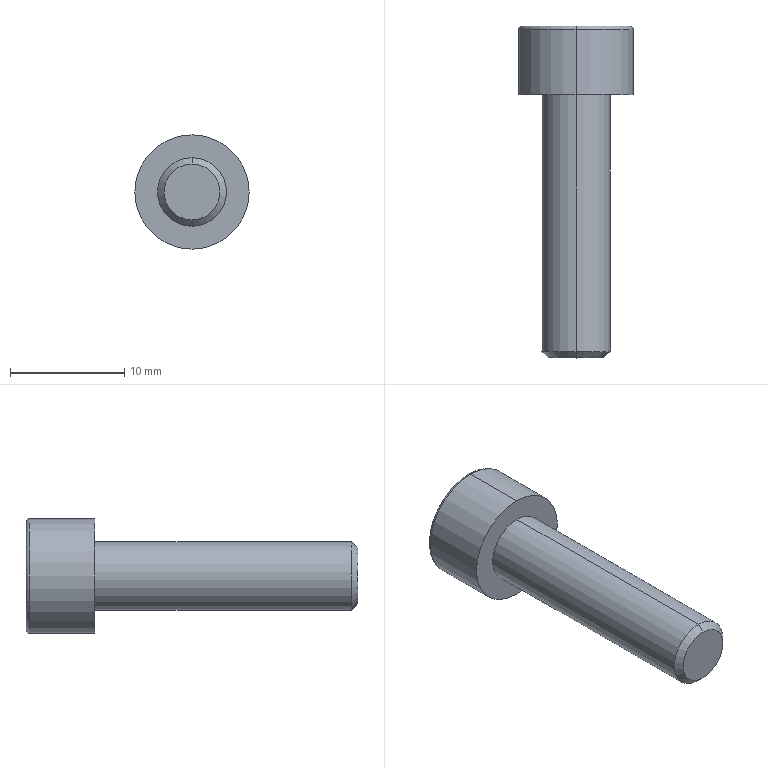Part | SolidWorks | features BaseBody 1 | 1 solid | 18 faces | box 10 x 29 x 10 mm | volume 1051 mm3 | plane 10 | cylinder 4 | cone 2 | torus 2 | commonest cylinder face diameters 6 x2 10 x2
STEP:
#1=CARTESIAN_POINT('',(0.,-23.,-2.445));
#2=VERTEX_POINT('',#1);
#3=CARTESIAN_POINT('',(0.,-23.,2.445));
#4=VERTEX_POINT('',#3);
#5=CARTESIAN_POINT('',(0.,-23.,0.));
#6=DIRECTION('',(0.,-1.,0.));
#7=DIRECTION('',(0.,0.,-1.));
#8=AXIS2_PLACEMENT_3D('',#5,#6,#7);
#9=CIRCLE('',#8,2.445);
#10=EDGE_CURVE('',#2,#4,#9,.T.);
#11=ORIENTED_EDGE('',*,*,#10,.F.);
#12=CARTESIAN_POINT('',(0.,-22.445,-3.));
#13=VERTEX_POINT('',#12);
#14=CARTESIAN_POINT('',(0.,-23.,-2.445));
#15=DIRECTION('',(0.,0.7071,-0.7071));
#16=VECTOR('',#15,1000.);
#17=LINE('',#14,#16);
#18=EDGE_CURVE('',#2,#13,#17,.T.);
#19=ORIENTED_EDGE('',*,*,#18,.T.);
#20=CARTESIAN_POINT('',(0.,-22.445,3.));
#21=VERTEX_POINT('',#20);
#22=CARTESIAN_POINT('',(0.,-22.445,0.));
#23=DIRECTION('',(0.,1.,0.));
#24=DIRECTION('',(0.,0.,-1.));
#25=AXIS2_PLACEMENT_3D('',#22,#23,#24);
#26=CIRCLE('',#25,3.);
#27=EDGE_CURVE('',#21,#13,#26,.T.);
#28=ORIENTED_EDGE('',*,*,#27,.F.);
#29=CARTESIAN_POINT('',(0.,-23.,2.445));
#30=DIRECTION('',(0.,0.7071,0.7071));
#31=VECTOR('',#30,1000.);
#32=LINE('',#29,#31);
#33=EDGE_CURVE('',#4,#21,#32,.T.);
#34=ORIENTED_EDGE('',*,*,#33,.F.);
#35=EDGE_LOOP('',(#11,#19,#28,#34));
#36=FACE_OUTER_BOUND('',#35,.T.);
#37=CARTESIAN_POINT('',(0.,-23.,0.));
#38=DIRECTION('',(0.,1.,0.));
#39=DIRECTION('',(0.,0.,1.));
#40=AXIS2_PLACEMENT_3D('',#37,#38,#39);
#41=CONICAL_SURFACE('',#40,2.445,0.7854);
#42=ADVANCED_FACE('',(#36),#41,.T.);
#43=ORIENTED_EDGE('',*,*,#27,.T.);
#44=CARTESIAN_POINT('',(0.,0.,-3.));
#45=VERTEX_POINT('',#44);
#46=CARTESIAN_POINT('',(0.,-23.,-3.));
#47=DIRECTION('',(0.,1.,0.));
#48=VECTOR('',#47,1000.);
#49=LINE('',#46,#48);
#50=EDGE_CURVE('',#13,#45,#49,.T.);
#51=ORIENTED_EDGE('',*,*,#50,.T.);
#52=CARTESIAN_POINT('',(0.,0.,3.));
#53=VERTEX_POINT('',#52);
#54=CARTESIAN_POINT('',(0.,0.,0.));
#55=DIRECTION('',(0.,-1.,0.));
#56=DIRECTION('',(0.,0.,1.));
#57=AXIS2_PLACEMENT_3D('',#54,#55,#56);
#58=CIRCLE('',#57,3.);
#59=EDGE_CURVE('',#45,#53,#58,.T.);
#60=ORIENTED_EDGE('',*,*,#59,.T.);
#61=CARTESIAN_POINT('',(0.,-23.,3.));
#62=DIRECTION('',(0.,1.,0.));
#63=VECTOR('',#62,1000.);
#64=LINE('',#61,#63);
#65=EDGE_CURVE('',#21,#53,#64,.T.);
#66=ORIENTED_EDGE('',*,*,#65,.F.);
#67=EDGE_LOOP('',(#43,#51,#60,#66));
#68=FACE_OUTER_BOUND('',#67,.T.);
#69=CARTESIAN_POINT('',(0.,-23.,0.));
#70=DIRECTION('',(0.,1.,0.));
#71=DIRECTION('',(0.,0.,1.));
#72=AXIS2_PLACEMENT_3D('',#69,#70,#71);
#73=CYLINDRICAL_SURFACE('',#72,3.);
#74=ADVANCED_FACE('',(#68),#73,.T.);
#75=CARTESIAN_POINT('',(0.,5.7,-5.));
#76=VERTEX_POINT('',#75);
#77=CARTESIAN_POINT('',(0.,5.7,5.));
#78=VERTEX_POINT('',#77);
#79=CARTESIAN_POINT('',(0.,5.7,0.));
#80=DIRECTION('',(0.,-1.,0.));
#81=DIRECTION('',(0.,0.,1.));
#82=AXIS2_PLACEMENT_3D('',#79,#80,#81);
#83=CIRCLE('',#82,5.);
#84=EDGE_CURVE('',#76,#78,#83,.T.);
#85=ORIENTED_EDGE('',*,*,#84,.F.);
#86=CARTESIAN_POINT('',(0.,6.,-4.7));
#87=VERTEX_POINT('',#86);
#88=CARTESIAN_POINT('',(0.,5.7,-4.7));
#89=DIRECTION('',(1.,0.,0.));
#90=DIRECTION('',(0.,0.,-1.));
#91=AXIS2_PLACEMENT_3D('',#88,#89,#90);
#92=CIRCLE('',#91,0.3);
#93=EDGE_CURVE('',#76,#87,#92,.T.);
#94=ORIENTED_EDGE('',*,*,#93,.T.);
#95=CARTESIAN_POINT('',(0.,6.,4.7));
#96=VERTEX_POINT('',#95);
#97=CARTESIAN_POINT('',(0.,6.,0.));
#98=DIRECTION('',(0.,1.,0.));
#99=DIRECTION('',(0.,0.,1.));
#100=AXIS2_PLACEMENT_3D('',#97,#98,#99);
#101=CIRCLE('',#100,4.7);
#102=EDGE_CURVE('',#96,#87,#101,.T.);
#103=ORIENTED_EDGE('',*,*,#102,.F.);
#104=CARTESIAN_POINT('',(0.,5.7,4.7));
#105=DIRECTION('',(-1.,0.,0.));
#106=DIRECTION('',(0.,0.,1.));
#107=AXIS2_PLACEMENT_3D('',#104,#105,#106);
#108=CIRCLE('',#107,0.3);
#109=EDGE_CURVE('',#78,#96,#108,.T.);
#110=ORIENTED_EDGE('',*,*,#109,.F.);
#111=EDGE_LOOP('',(#85,#94,#103,#110));
#112=FACE_OUTER_BOUND('',#111,.T.);
#113=CARTESIAN_POINT('',(0.,5.7,0.));
#114=DIRECTION('',(0.,1.,0.));
#115=DIRECTION('',(0.,0.,1.));
#116=AXIS2_PLACEMENT_3D('',#113,#114,#115);
#117=TOROIDAL_SURFACE('',#116,4.7,0.3);
#118=ADVANCED_FACE('',(#112),#117,.T.);
#119=ORIENTED_EDGE('',*,*,#84,.T.);
#120=CARTESIAN_POINT('',(0.,0.,5.));
#121=VERTEX_POINT('',#120);
#122=CARTESIAN_POINT('',(0.,6.,5.));
#123=DIRECTION('',(0.,-1.,0.));
#124=VECTOR('',#123,1000.);
#125=LINE('',#122,#124);
#126=EDGE_CURVE('',#78,#121,#125,.T.);
#127=ORIENTED_EDGE('',*,*,#126,.T.);
#128=CARTESIAN_POINT('',(0.,0.,-5.));
#129=VERTEX_POINT('',#128);
#130=CARTESIAN_POINT('',(0.,0.,0.));
#131=DIRECTION('',(0.,1.,0.));
#132=DIRECTION('',(0.,0.,1.));
#133=AXIS2_PLACEMENT_3D('',#130,#131,#132);
#134=CIRCLE('',#133,5.);
#135=EDGE_CURVE('',#121,#129,#134,.T.);
#136=ORIENTED_EDGE('',*,*,#135,.T.);
#137=CARTESIAN_POINT('',(0.,6.,-5.));
#138=DIRECTION('',(0.,-1.,0.));
#139=VECTOR('',#138,1000.);
#140=LINE('',#137,#139);
#141=EDGE_CURVE('',#76,#129,#140,.T.);
#142=ORIENTED_EDGE('',*,*,#141,.F.);
#143=EDGE_LOOP('',(#119,#127,#136,#142));
#144=FACE_OUTER_BOUND('',#143,.T.);
#145=CARTESIAN_POINT('',(0.,6.,0.));
#146=DIRECTION('',(0.,-1.,0.));
#147=DIRECTION('',(0.,0.,-1.));
#148=AXIS2_PLACEMENT_3D('',#145,#146,#147);
#149=CYLINDRICAL_SURFACE('',#148,5.);
#150=ADVANCED_FACE('',(#144),#149,.T.);
#151=CARTESIAN_POINT('',(0.,-23.,0.));
#152=DIRECTION('',(0.,-1.,0.));
#153=DIRECTION('',(0.,0.,-1.));
#154=AXIS2_PLACEMENT_3D('',#151,#152,#153);
#155=CIRCLE('',#154,2.445);
#156=EDGE_CURVE('',#4,#2,#155,.T.);
#157=ORIENTED_EDGE('',*,*,#156,.T.);
#158=ORIENTED_EDGE('',*,*,#10,.T.);
#159=EDGE_LOOP('',(#157,#158));
#160=FACE_OUTER_BOUND('',#159,.T.);
#161=CARTESIAN_POINT('',(0.,-23.,0.));
#162=DIRECTION('',(0.,-1.,0.));
#163=DIRECTION('',(0.,0.,-1.));
#164=AXIS2_PLACEMENT_3D('',#161,#162,#163);
#165=PLANE('',#164);
#166=ADVANCED_FACE('',(#160),#165,.T.);
#167=CARTESIAN_POINT('',(1.466,3.,2.54));
#168=VERTEX_POINT('',#167);
#169=CARTESIAN_POINT('',(2.933,3.,0.));
#170=VERTEX_POINT('',#169);
#171=CARTESIAN_POINT('',(1.466,3.,2.54));
#172=DIRECTION('',(0.5,0.,-0.866));
#173=VECTOR('',#172,1000.);
#174=LINE('',#171,#173);
#175=EDGE_CURVE('',#168,#170,#174,.T.);
#176=ORIENTED_EDGE('',*,*,#175,.T.);
#177=CARTESIAN_POINT('',(1.466,3.,-2.54));
#178=VERTEX_POINT('',#177);
#179=CARTESIAN_POINT('',(2.933,3.,0.));
#180=DIRECTION('',(-0.5,0.,-0.866));
#181=VECTOR('',#180,1000.);
#182=LINE('',#179,#181);
#183=EDGE_CURVE('',#170,#178,#182,.T.);
#184=ORIENTED_EDGE('',*,*,#183,.T.);
#185=CARTESIAN_POINT('',(-1.466,3.,-2.54));
#186=VERTEX_POINT('',#185);
#187=CARTESIAN_POINT('',(1.466,3.,-2.54));
#188=DIRECTION('',(-1.,0.,0.));
#189=VECTOR('',#188,1000.);
#190=LINE('',#187,#189);
#191=EDGE_CURVE('',#178,#186,#190,.T.);
#192=ORIENTED_EDGE('',*,*,#191,.T.);
#193=CARTESIAN_POINT('',(-2.933,3.,0.));
#194=VERTEX_POINT('',#193);
#195=CARTESIAN_POINT('',(-1.466,3.,-2.54));
#196=DIRECTION('',(-0.5,0.,0.866));
#197=VECTOR('',#196,1000.);
#198=LINE('',#195,#197);
#199=EDGE_CURVE('',#186,#194,#198,.T.);
#200=ORIENTED_EDGE('',*,*,#199,.T.);
#201=CARTESIAN_POINT('',(-1.466,3.,2.54));
#202=VERTEX_POINT('',#201);
#203=CARTESIAN_POINT('',(-2.933,3.,0.));
#204=DIRECTION('',(0.5,0.,0.866));
#205=VECTOR('',#204,1000.);
#206=LINE('',#203,#205);
#207=EDGE_CURVE('',#194,#202,#206,.T.);
#208=ORIENTED_EDGE('',*,*,#207,.T.);
#209=CARTESIAN_POINT('',(-1.466,3.,2.54));
#210=DIRECTION('',(1.,0.,0.));
#211=VECTOR('',#210,1000.);
#212=LINE('',#209,#211);
#213=EDGE_CURVE('',#202,#168,#212,.T.);
#214=ORIENTED_EDGE('',*,*,#213,.T.);
#215=EDGE_LOOP('',(#176,#184,#192,#200,#208,#214));
#216=FACE_OUTER_BOUND('',#215,.T.);
#217=CARTESIAN_POINT('',(0.,3.,0.));
#218=DIRECTION('',(0.,1.,0.));
#219=DIRECTION('',(1.,0.,0.));
#220=AXIS2_PLACEMENT_3D('',#217,#218,#219);
#221=PLANE('',#220);
#222=ADVANCED_FACE('',(#216),#221,.T.);
#223=CARTESIAN_POINT('',(2.933,6.,0.));
#224=VERTEX_POINT('',#223);
#225=CARTESIAN_POINT('',(1.466,6.,-2.54));
#226=VERTEX_POINT('',#225);
#227=CARTESIAN_POINT('',(2.933,6.,0.));
#228=DIRECTION('',(-0.5,0.,-0.866));
#229=VECTOR('',#228,1000.);
#230=LINE('',#227,#229);
#231=EDGE_CURVE('',#224,#226,#230,.T.);
#232=ORIENTED_EDGE('',*,*,#231,.T.);
#233=CARTESIAN_POINT('',(1.466,3.,-2.54));
#234=DIRECTION('',(0.,1.,0.));
#235=VECTOR('',#234,1000.);
#236=LINE('',#233,#235);
#237=EDGE_CURVE('',#178,#226,#236,.T.);
#238=ORIENTED_EDGE('',*,*,#237,.F.);
#239=ORIENTED_EDGE('',*,*,#183,.F.);
#240=CARTESIAN_POINT('',(2.933,3.,0.));
#241=DIRECTION('',(0.,1.,0.));
#242=VECTOR('',#241,1000.);
#243=LINE('',#240,#242);
#244=EDGE_CURVE('',#170,#224,#243,.T.);
#245=ORIENTED_EDGE('',*,*,#244,.T.);
#246=EDGE_LOOP('',(#232,#238,#239,#245));
#247=FACE_OUTER_BOUND('',#246,.T.);
#248=CARTESIAN_POINT('',(2.933,3.,0.));
#249=DIRECTION('',(0.866,0.,-0.5));
#250=DIRECTION('',(0.,-1.,0.));
#251=AXIS2_PLACEMENT_3D('',#248,#249,#250);
#252=PLANE('',#251);
#253=ADVANCED_FACE('',(#247),#252,.F.);
#254=CARTESIAN_POINT('',(-1.466,6.,-2.54));
#255=VERTEX_POINT('',#254);
#256=CARTESIAN_POINT('',(1.466,6.,-2.54));
#257=DIRECTION('',(-1.,0.,0.));
#258=VECTOR('',#257,1000.);
#259=LINE('',#256,#258);
#260=EDGE_CURVE('',#226,#255,#259,.T.);
#261=ORIENTED_EDGE('',*,*,#260,.T.);
#262=CARTESIAN_POINT('',(-1.466,3.,-2.54));
#263=DIRECTION('',(0.,1.,0.));
#264=VECTOR('',#263,1000.);
#265=LINE('',#262,#264);
#266=EDGE_CURVE('',#186,#255,#265,.T.);
#267=ORIENTED_EDGE('',*,*,#266,.F.);
#268=ORIENTED_EDGE('',*,*,#191,.F.);
#269=ORIENTED_EDGE('',*,*,#237,.T.);
#270=EDGE_LOOP('',(#261,#267,#268,#269));
#271=FACE_OUTER_BOUND('',#270,.T.);
#272=CARTESIAN_POINT('',(1.466,3.,-2.54));
#273=DIRECTION('',(0.,0.,-1.));
#274=DIRECTION('',(0.,-1.,0.));
#275=AXIS2_PLACEMENT_3D('',#272,#273,#274);
#276=PLANE('',#275);
#277=ADVANCED_FACE('',(#271),#276,.F.);
#278=CARTESIAN_POINT('',(-2.933,6.,0.));
#279=VERTEX_POINT('',#278);
#280=CARTESIAN_POINT('',(-1.466,6.,-2.54));
#281=DIRECTION('',(-0.5,0.,0.866));
#282=VECTOR('',#281,1000.);
#283=LINE('',#280,#282);
#284=EDGE_CURVE('',#255,#279,#283,.T.);
#285=ORIENTED_EDGE('',*,*,#284,.T.);
#286=CARTESIAN_POINT('',(-2.933,3.,0.));
#287=DIRECTION('',(0.,1.,0.));
#288=VECTOR('',#287,1000.);
#289=LINE('',#286,#288);
#290=EDGE_CURVE('',#194,#279,#289,.T.);
#291=ORIENTED_EDGE('',*,*,#290,.F.);
#292=ORIENTED_EDGE('',*,*,#199,.F.);
#293=ORIENTED_EDGE('',*,*,#266,.T.);
#294=EDGE_LOOP('',(#285,#291,#292,#293));
#295=FACE_OUTER_BOUND('',#294,.T.);
#296=CARTESIAN_POINT('',(-1.466,3.,-2.54));
#297=DIRECTION('',(-0.866,0.,-0.5));
#298=DIRECTION('',(-0.5,0.,0.866));
#299=AXIS2_PLACEMENT_3D('',#296,#297,#298);
#300=PLANE('',#299);
#301=ADVANCED_FACE('',(#295),#300,.F.);
#302=CARTESIAN_POINT('',(-1.466,6.,2.54));
#303=VERTEX_POINT('',#302);
#304=CARTESIAN_POINT('',(-2.933,6.,0.));
#305=DIRECTION('',(0.5,0.,0.866));
#306=VECTOR('',#305,1000.);
#307=LINE('',#304,#306);
#308=EDGE_CURVE('',#279,#303,#307,.T.);
#309=ORIENTED_EDGE('',*,*,#308,.T.);
#310=CARTESIAN_POINT('',(-1.466,3.,2.54));
#311=DIRECTION('',(0.,1.,0.));
#312=VECTOR('',#311,1000.);
#313=LINE('',#310,#312);
#314=EDGE_CURVE('',#202,#303,#313,.T.);
#315=ORIENTED_EDGE('',*,*,#314,.F.);
#316=ORIENTED_EDGE('',*,*,#207,.F.);
#317=ORIENTED_EDGE('',*,*,#290,.T.);
#318=EDGE_LOOP('',(#309,#315,#316,#317));
#319=FACE_OUTER_BOUND('',#318,.T.);
#320=CARTESIAN_POINT('',(-2.933,3.,0.));
#321=DIRECTION('',(-0.866,0.,0.5));
#322=DIRECTION('',(0.,1.,0.));
#323=AXIS2_PLACEMENT_3D('',#320,#321,#322);
#324=PLANE('',#323);
#325=ADVANCED_FACE('',(#319),#324,.F.);
#326=CARTESIAN_POINT('',(1.466,6.,2.54));
#327=VERTEX_POINT('',#326);
#328=CARTESIAN_POINT('',(-1.466,6.,2.54));
#329=DIRECTION('',(1.,0.,0.));
#330=VECTOR('',#329,1000.);
#331=LINE('',#328,#330);
#332=EDGE_CURVE('',#303,#327,#331,.T.);
#333=ORIENTED_EDGE('',*,*,#332,.T.);
#334=CARTESIAN_POINT('',(1.466,3.,2.54));
#335=DIRECTION('',(0.,1.,0.));
#336=VECTOR('',#335,1000.);
#337=LINE('',#334,#336);
#338=EDGE_CURVE('',#168,#327,#337,.T.);
#339=ORIENTED_EDGE('',*,*,#338,.F.);
#340=ORIENTED_EDGE('',*,*,#213,.F.);
#341=ORIENTED_EDGE('',*,*,#314,.T.);
#342=EDGE_LOOP('',(#333,#339,#340,#341));
#343=FACE_OUTER_BOUND('',#342,.T.);
#344=CARTESIAN_POINT('',(-1.466,3.,2.54));
#345=DIRECTION('',(0.,0.,1.));
#346=DIRECTION('',(1.,0.,0.));
#347=AXIS2_PLACEMENT_3D('',#344,#345,#346);
#348=PLANE('',#347);
#349=ADVANCED_FACE('',(#343),#348,.F.);
#350=CARTESIAN_POINT('',(1.466,6.,2.54));
#351=DIRECTION('',(0.5,0.,-0.866));
#352=VECTOR('',#351,1000.);
#353=LINE('',#350,#352);
#354=EDGE_CURVE('',#327,#224,#353,.T.);
#355=ORIENTED_EDGE('',*,*,#354,.T.);
#356=ORIENTED_EDGE('',*,*,#244,.F.);
#357=ORIENTED_EDGE('',*,*,#175,.F.);
#358=ORIENTED_EDGE('',*,*,#338,.T.);
#359=EDGE_LOOP('',(#355,#356,#357,#358));
#360=FACE_OUTER_BOUND('',#359,.T.);
#361=CARTESIAN_POINT('',(1.466,3.,2.54));
#362=DIRECTION('',(0.866,0.,0.5));
#363=DIRECTION('',(0.,-1.,0.));
#364=AXIS2_PLACEMENT_3D('',#361,#362,#363);
#365=PLANE('',#364);
#366=ADVANCED_FACE('',(#360),#365,.F.);
#367=ORIENTED_EDGE('',*,*,#354,.F.);
#368=ORIENTED_EDGE('',*,*,#332,.F.);
#369=ORIENTED_EDGE('',*,*,#308,.F.);
#370=ORIENTED_EDGE('',*,*,#284,.F.);
#371=ORIENTED_EDGE('',*,*,#260,.F.);
#372=ORIENTED_EDGE('',*,*,#231,.F.);
#373=EDGE_LOOP('',(#367,#368,#369,#370,#371,#372));
#374=FACE_BOUND('',#373,.T.);
#375=ORIENTED_EDGE('',*,*,#102,.T.);
#376=CARTESIAN_POINT('',(0.,6.,0.));
#377=DIRECTION('',(0.,1.,0.));
#378=DIRECTION('',(0.,0.,1.));
#379=AXIS2_PLACEMENT_3D('',#376,#377,#378);
#380=CIRCLE('',#379,4.7);
#381=EDGE_CURVE('',#87,#96,#380,.T.);
#382=ORIENTED_EDGE('',*,*,#381,.T.);
#383=EDGE_LOOP('',(#375,#382));
#384=FACE_OUTER_BOUND('',#383,.T.);
#385=CARTESIAN_POINT('',(0.,6.,0.));
#386=DIRECTION('',(0.,1.,0.));
#387=DIRECTION('',(1.,0.,0.));
#388=AXIS2_PLACEMENT_3D('',#385,#386,#387);
#389=PLANE('',#388);
#390=ADVANCED_FACE('',(#374,#384),#389,.T.);
#391=CARTESIAN_POINT('',(0.,0.,0.));
#392=DIRECTION('',(0.,-1.,0.));
#393=DIRECTION('',(0.,0.,1.));
#394=AXIS2_PLACEMENT_3D('',#391,#392,#393);
#395=CIRCLE('',#394,3.);
#396=EDGE_CURVE('',#53,#45,#395,.T.);
#397=ORIENTED_EDGE('',*,*,#396,.F.);
#398=ORIENTED_EDGE('',*,*,#59,.F.);
#399=EDGE_LOOP('',(#397,#398));
#400=FACE_BOUND('',#399,.T.);
#401=CARTESIAN_POINT('',(0.,0.,0.));
#402=DIRECTION('',(0.,1.,0.));
#403=DIRECTION('',(0.,0.,1.));
#404=AXIS2_PLACEMENT_3D('',#401,#402,#403);
#405=CIRCLE('',#404,5.);
#406=EDGE_CURVE('',#129,#121,#405,.T.);
#407=ORIENTED_EDGE('',*,*,#406,.F.);
#408=ORIENTED_EDGE('',*,*,#135,.F.);
#409=EDGE_LOOP('',(#407,#408));
#410=FACE_OUTER_BOUND('',#409,.T.);
#411=CARTESIAN_POINT('',(0.,0.,0.));
#412=DIRECTION('',(0.,1.,0.));
#413=DIRECTION('',(1.,0.,0.));
#414=AXIS2_PLACEMENT_3D('',#411,#412,#413);
#415=PLANE('',#414);
#416=ADVANCED_FACE('',(#400,#410),#415,.F.);
#417=ORIENTED_EDGE('',*,*,#126,.F.);
#418=CARTESIAN_POINT('',(0.,5.7,0.));
#419=DIRECTION('',(0.,-1.,0.));
#420=DIRECTION('',(0.,0.,1.));
#421=AXIS2_PLACEMENT_3D('',#418,#419,#420);
#422=CIRCLE('',#421,5.);
#423=EDGE_CURVE('',#78,#76,#422,.T.);
#424=ORIENTED_EDGE('',*,*,#423,.T.);
#425=ORIENTED_EDGE('',*,*,#141,.T.);
#426=ORIENTED_EDGE('',*,*,#406,.T.);
#427=EDGE_LOOP('',(#417,#424,#425,#426));
#428=FACE_OUTER_BOUND('',#427,.T.);
#429=CARTESIAN_POINT('',(0.,6.,0.));
#430=DIRECTION('',(0.,-1.,0.));
#431=DIRECTION('',(0.,0.,-1.));
#432=AXIS2_PLACEMENT_3D('',#429,#430,#431);
#433=CYLINDRICAL_SURFACE('',#432,5.);
#434=ADVANCED_FACE('',(#428),#433,.T.);
#435=ORIENTED_EDGE('',*,*,#93,.F.);
#436=ORIENTED_EDGE('',*,*,#423,.F.);
#437=ORIENTED_EDGE('',*,*,#109,.T.);
#438=ORIENTED_EDGE('',*,*,#381,.F.);
#439=EDGE_LOOP('',(#435,#436,#437,#438));
#440=FACE_OUTER_BOUND('',#439,.T.);
#441=CARTESIAN_POINT('',(0.,5.7,0.));
#442=DIRECTION('',(0.,1.,0.));
#443=DIRECTION('',(0.,0.,1.));
#444=AXIS2_PLACEMENT_3D('',#441,#442,#443);
#445=TOROIDAL_SURFACE('',#444,4.7,0.3);
#446=ADVANCED_FACE('',(#440),#445,.T.);
#447=ORIENTED_EDGE('',*,*,#50,.F.);
#448=CARTESIAN_POINT('',(0.,-22.445,0.));
#449=DIRECTION('',(0.,1.,0.));
#450=DIRECTION('',(0.,0.,-1.));
#451=AXIS2_PLACEMENT_3D('',#448,#449,#450);
#452=CIRCLE('',#451,3.);
#453=EDGE_CURVE('',#13,#21,#452,.T.);
#454=ORIENTED_EDGE('',*,*,#453,.T.);
#455=ORIENTED_EDGE('',*,*,#65,.T.);
#456=ORIENTED_EDGE('',*,*,#396,.T.);
#457=EDGE_LOOP('',(#447,#454,#455,#456));
#458=FACE_OUTER_BOUND('',#457,.T.);
#459=CARTESIAN_POINT('',(0.,-23.,0.));
#460=DIRECTION('',(0.,1.,0.));
#461=DIRECTION('',(0.,0.,1.));
#462=AXIS2_PLACEMENT_3D('',#459,#460,#461);
#463=CYLINDRICAL_SURFACE('',#462,3.);
#464=ADVANCED_FACE('',(#458),#463,.T.);
#465=ORIENTED_EDGE('',*,*,#18,.F.);
#466=ORIENTED_EDGE('',*,*,#156,.F.);
#467=ORIENTED_EDGE('',*,*,#33,.T.);
#468=ORIENTED_EDGE('',*,*,#453,.F.);
#469=EDGE_LOOP('',(#465,#466,#467,#468));
#470=FACE_OUTER_BOUND('',#469,.T.);
#471=CARTESIAN_POINT('',(0.,-23.,0.));
#472=DIRECTION('',(0.,1.,0.));
#473=DIRECTION('',(0.,0.,1.));
#474=AXIS2_PLACEMENT_3D('',#471,#472,#473);
#475=CONICAL_SURFACE('',#474,2.445,0.7854);
#476=ADVANCED_FACE('',(#470),#475,.T.);
#477=CLOSED_SHELL('',(#42,#74,#118,#150,#166,#222,#253,#277,#301,#325,#349,#366,#390,#416,#434,#446,#464,#476));
#478=MANIFOLD_SOLID_BREP('',#477);
#479=CARTESIAN_POINT('',(0.,0.,0.));
#480=DIRECTION('',(0.,0.,1.));
#481=DIRECTION('',(1.,0.,0.));
#482=AXIS2_PLACEMENT_3D('',#479,#480,#481);
#483=(LENGTH_UNIT()NAMED_UNIT(*)SI_UNIT(.MILLI.,.METRE.));
#484=UNCERTAINTY_MEASURE_WITH_UNIT(LENGTH_MEASURE(0.00001),#483,'','');
#485=(NAMED_UNIT(*)PLANE_ANGLE_UNIT()SI_UNIT($,.RADIAN.));
#486=(NAMED_UNIT(*)SI_UNIT($,.STERADIAN.)SOLID_ANGLE_UNIT());
#487=(GEOMETRIC_REPRESENTATION_CONTEXT(3)GLOBAL_UNCERTAINTY_ASSIGNED_CONTEXT((#484))GLOBAL_UNIT_ASSIGNED_CONTEXT((#483,#485,#486))REPRESENTATION_CONTEXT('',''));
#488=ADVANCED_BREP_SHAPE_REPRESENTATION('',(#478,#482),#487);